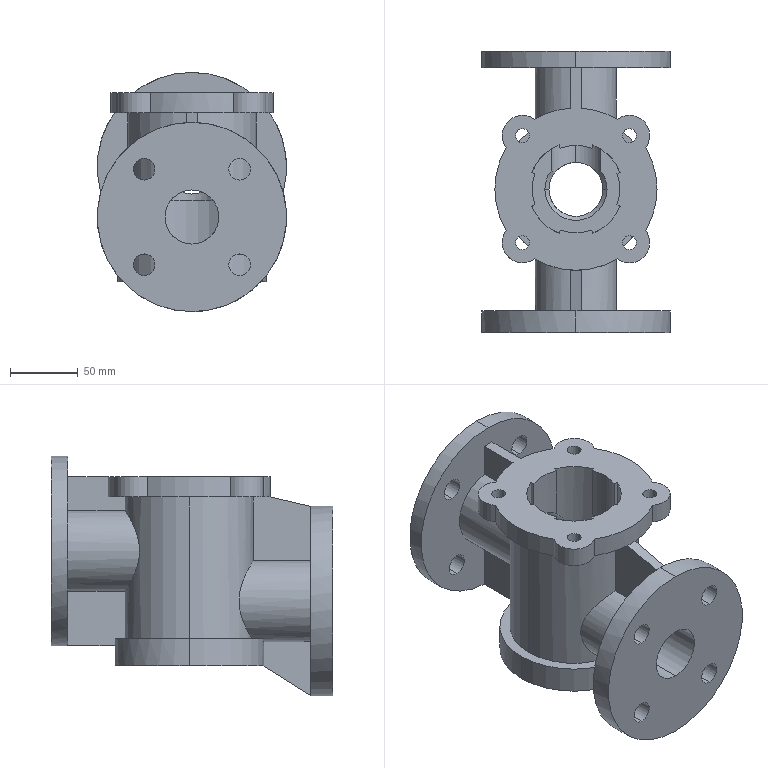Part | SolidWorks | features ICE 14, RevCut 3, 3DProfileFeature 1, Chamfer 1, CirPattern 1, CombineBodies 1, Extrusion 1, HoleWzd 1, Split 1 | 1 solid | 132 faces | box 140 x 208 x 177 mm | volume 1195368 mm3 | cylinder 76 | plane 45 | cone 11 | commonest cylinder face diameters 10.3 x16 16 x16 40 x8 30 x6 120 x6 65 x5